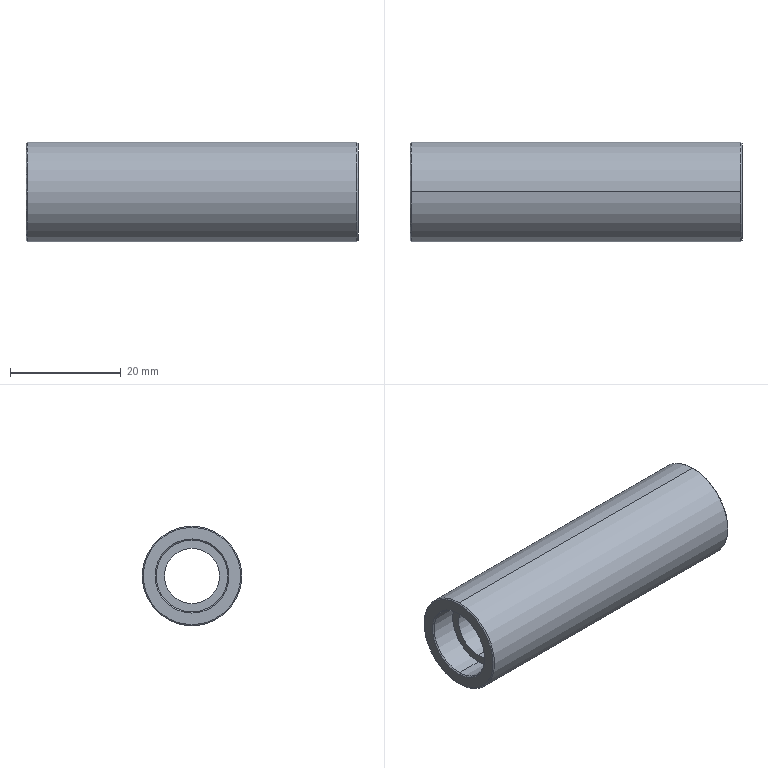Part | SolidWorks | features Chamfer 1, Revolution 1 | 1 solid | 20 faces | box 60 x 18 x 18 mm | volume 10010 mm3 | cone 8 | cylinder 8 | plane 4 | commonest cylinder face diameters 13 x4 10 x2 18 x2
STEP:
#1=CARTESIAN_POINT('',(59.8,0.,6.5));
#2=VERTEX_POINT('',#1);
#3=CARTESIAN_POINT('',(59.8,0.,-6.5));
#4=VERTEX_POINT('',#3);
#5=CARTESIAN_POINT('',(59.8,0.,0.));
#6=DIRECTION('',(1.,0.,0.));
#7=DIRECTION('',(0.,0.,1.));
#8=AXIS2_PLACEMENT_3D('',#5,#6,#7);
#9=CIRCLE('',#8,6.5);
#10=EDGE_CURVE('',#2,#4,#9,.T.);
#11=ORIENTED_EDGE('',*,*,#10,.F.);
#12=CARTESIAN_POINT('',(60.,0.,6.7));
#13=VERTEX_POINT('',#12);
#14=CARTESIAN_POINT('',(60.,0.,6.7));
#15=DIRECTION('',(0.7071,0.,0.7071));
#16=VECTOR('',#15,1000.);
#17=LINE('',#14,#16);
#18=EDGE_CURVE('',#2,#13,#17,.T.);
#19=ORIENTED_EDGE('',*,*,#18,.T.);
#20=CARTESIAN_POINT('',(60.,0.,-6.7));
#21=VERTEX_POINT('',#20);
#22=CARTESIAN_POINT('',(60.,0.,0.));
#23=DIRECTION('',(-1.,0.,0.));
#24=DIRECTION('',(0.,0.,1.));
#25=AXIS2_PLACEMENT_3D('',#22,#23,#24);
#26=CIRCLE('',#25,6.7);
#27=EDGE_CURVE('',#21,#13,#26,.T.);
#28=ORIENTED_EDGE('',*,*,#27,.F.);
#29=CARTESIAN_POINT('',(60.,0.,-6.7));
#30=DIRECTION('',(0.7071,0.,-0.7071));
#31=VECTOR('',#30,1000.);
#32=LINE('',#29,#31);
#33=EDGE_CURVE('',#4,#21,#32,.T.);
#34=ORIENTED_EDGE('',*,*,#33,.F.);
#35=EDGE_LOOP('',(#11,#19,#28,#34));
#36=FACE_OUTER_BOUND('',#35,.T.);
#37=CARTESIAN_POINT('',(60.,0.,0.));
#38=DIRECTION('',(1.,0.,0.));
#39=DIRECTION('',(0.,0.,-1.));
#40=AXIS2_PLACEMENT_3D('',#37,#38,#39);
#41=CONICAL_SURFACE('',#40,6.7,0.7854);
#42=ADVANCED_FACE('',(#36),#41,.F.);
#43=CARTESIAN_POINT('',(60.,0.,-8.8));
#44=VERTEX_POINT('',#43);
#45=CARTESIAN_POINT('',(60.,0.,8.8));
#46=VERTEX_POINT('',#45);
#47=CARTESIAN_POINT('',(60.,0.,0.));
#48=DIRECTION('',(1.,0.,0.));
#49=DIRECTION('',(0.,0.,1.));
#50=AXIS2_PLACEMENT_3D('',#47,#48,#49);
#51=CIRCLE('',#50,8.8);
#52=EDGE_CURVE('',#44,#46,#51,.T.);
#53=ORIENTED_EDGE('',*,*,#52,.F.);
#54=CARTESIAN_POINT('',(59.8,0.,-9.));
#55=VERTEX_POINT('',#54);
#56=CARTESIAN_POINT('',(59.8,0.,-9.));
#57=DIRECTION('',(-0.7071,0.,-0.7071));
#58=VECTOR('',#57,1000.);
#59=LINE('',#56,#58);
#60=EDGE_CURVE('',#44,#55,#59,.T.);
#61=ORIENTED_EDGE('',*,*,#60,.T.);
#62=CARTESIAN_POINT('',(59.8,0.,9.));
#63=VERTEX_POINT('',#62);
#64=CARTESIAN_POINT('',(59.8,0.,0.));
#65=DIRECTION('',(-1.,0.,0.));
#66=DIRECTION('',(0.,0.,1.));
#67=AXIS2_PLACEMENT_3D('',#64,#65,#66);
#68=CIRCLE('',#67,9.);
#69=EDGE_CURVE('',#63,#55,#68,.T.);
#70=ORIENTED_EDGE('',*,*,#69,.F.);
#71=CARTESIAN_POINT('',(59.8,0.,9.));
#72=DIRECTION('',(-0.7071,0.,0.7071));
#73=VECTOR('',#72,1000.);
#74=LINE('',#71,#73);
#75=EDGE_CURVE('',#46,#63,#74,.T.);
#76=ORIENTED_EDGE('',*,*,#75,.F.);
#77=EDGE_LOOP('',(#53,#61,#70,#76));
#78=FACE_OUTER_BOUND('',#77,.T.);
#79=CARTESIAN_POINT('',(59.8,0.,0.));
#80=DIRECTION('',(-1.,0.,0.));
#81=DIRECTION('',(0.,0.,1.));
#82=AXIS2_PLACEMENT_3D('',#79,#80,#81);
#83=CONICAL_SURFACE('',#82,9.,0.7854);
#84=ADVANCED_FACE('',(#78),#83,.T.);
#85=CARTESIAN_POINT('',(0.2,0.,-6.5));
#86=VERTEX_POINT('',#85);
#87=CARTESIAN_POINT('',(0.2,0.,6.5));
#88=VERTEX_POINT('',#87);
#89=CARTESIAN_POINT('',(0.2,0.,0.));
#90=DIRECTION('',(-1.,0.,0.));
#91=DIRECTION('',(0.,0.,-1.));
#92=AXIS2_PLACEMENT_3D('',#89,#90,#91);
#93=CIRCLE('',#92,6.5);
#94=EDGE_CURVE('',#86,#88,#93,.T.);
#95=ORIENTED_EDGE('',*,*,#94,.F.);
#96=CARTESIAN_POINT('',(0.,0.,-6.7));
#97=VERTEX_POINT('',#96);
#98=CARTESIAN_POINT('',(0.2,0.,-6.5));
#99=DIRECTION('',(-0.7071,0.,-0.7071));
#100=VECTOR('',#99,1000.);
#101=LINE('',#98,#100);
#102=EDGE_CURVE('',#86,#97,#101,.T.);
#103=ORIENTED_EDGE('',*,*,#102,.T.);
#104=CARTESIAN_POINT('',(0.,0.,6.7));
#105=VERTEX_POINT('',#104);
#106=CARTESIAN_POINT('',(0.,0.,0.));
#107=DIRECTION('',(1.,0.,0.));
#108=DIRECTION('',(0.,0.,-1.));
#109=AXIS2_PLACEMENT_3D('',#106,#107,#108);
#110=CIRCLE('',#109,6.7);
#111=EDGE_CURVE('',#105,#97,#110,.T.);
#112=ORIENTED_EDGE('',*,*,#111,.F.);
#113=CARTESIAN_POINT('',(0.2,0.,6.5));
#114=DIRECTION('',(-0.7071,0.,0.7071));
#115=VECTOR('',#114,1000.);
#116=LINE('',#113,#115);
#117=EDGE_CURVE('',#88,#105,#116,.T.);
#118=ORIENTED_EDGE('',*,*,#117,.F.);
#119=EDGE_LOOP('',(#95,#103,#112,#118));
#120=FACE_OUTER_BOUND('',#119,.T.);
#121=CARTESIAN_POINT('',(0.2,0.,0.));
#122=DIRECTION('',(-1.,0.,0.));
#123=DIRECTION('',(0.,0.,1.));
#124=AXIS2_PLACEMENT_3D('',#121,#122,#123);
#125=CONICAL_SURFACE('',#124,6.5,0.7854);
#126=ADVANCED_FACE('',(#120),#125,.F.);
#127=CARTESIAN_POINT('',(0.,0.,8.8));
#128=VERTEX_POINT('',#127);
#129=CARTESIAN_POINT('',(0.,0.,-8.8));
#130=VERTEX_POINT('',#129);
#131=CARTESIAN_POINT('',(0.,0.,0.));
#132=DIRECTION('',(-1.,0.,0.));
#133=DIRECTION('',(0.,0.,-1.));
#134=AXIS2_PLACEMENT_3D('',#131,#132,#133);
#135=CIRCLE('',#134,8.8);
#136=EDGE_CURVE('',#128,#130,#135,.T.);
#137=ORIENTED_EDGE('',*,*,#136,.F.);
#138=CARTESIAN_POINT('',(0.2,0.,9.));
#139=VERTEX_POINT('',#138);
#140=CARTESIAN_POINT('',(0.,0.,8.8));
#141=DIRECTION('',(0.7071,0.,0.7071));
#142=VECTOR('',#141,1000.);
#143=LINE('',#140,#142);
#144=EDGE_CURVE('',#128,#139,#143,.T.);
#145=ORIENTED_EDGE('',*,*,#144,.T.);
#146=CARTESIAN_POINT('',(0.2,0.,-9.));
#147=VERTEX_POINT('',#146);
#148=CARTESIAN_POINT('',(0.2,0.,0.));
#149=DIRECTION('',(1.,0.,0.));
#150=DIRECTION('',(0.,0.,-1.));
#151=AXIS2_PLACEMENT_3D('',#148,#149,#150);
#152=CIRCLE('',#151,9.);
#153=EDGE_CURVE('',#147,#139,#152,.T.);
#154=ORIENTED_EDGE('',*,*,#153,.F.);
#155=CARTESIAN_POINT('',(0.,0.,-8.8));
#156=DIRECTION('',(0.7071,0.,-0.7071));
#157=VECTOR('',#156,1000.);
#158=LINE('',#155,#157);
#159=EDGE_CURVE('',#130,#147,#158,.T.);
#160=ORIENTED_EDGE('',*,*,#159,.F.);
#161=EDGE_LOOP('',(#137,#145,#154,#160));
#162=FACE_OUTER_BOUND('',#161,.T.);
#163=CARTESIAN_POINT('',(0.,0.,0.));
#164=DIRECTION('',(1.,0.,0.));
#165=DIRECTION('',(0.,0.,-1.));
#166=AXIS2_PLACEMENT_3D('',#163,#164,#165);
#167=CONICAL_SURFACE('',#166,8.8,0.7854);
#168=ADVANCED_FACE('',(#162),#167,.T.);
#169=CARTESIAN_POINT('',(5.,0.,-6.5));
#170=VERTEX_POINT('',#169);
#171=CARTESIAN_POINT('',(5.,0.,6.5));
#172=VERTEX_POINT('',#171);
#173=CARTESIAN_POINT('',(5.,0.,0.));
#174=DIRECTION('',(-1.,0.,0.));
#175=DIRECTION('',(0.,0.,1.));
#176=AXIS2_PLACEMENT_3D('',#173,#174,#175);
#177=CIRCLE('',#176,6.5);
#178=EDGE_CURVE('',#170,#172,#177,.T.);
#179=ORIENTED_EDGE('',*,*,#178,.F.);
#180=CARTESIAN_POINT('',(0.,0.,-6.5));
#181=DIRECTION('',(-1.,0.,0.));
#182=VECTOR('',#181,1000.);
#183=LINE('',#180,#182);
#184=EDGE_CURVE('',#170,#86,#183,.T.);
#185=ORIENTED_EDGE('',*,*,#184,.T.);
#186=ORIENTED_EDGE('',*,*,#94,.T.);
#187=CARTESIAN_POINT('',(0.,0.,6.5));
#188=DIRECTION('',(-1.,0.,0.));
#189=VECTOR('',#188,1000.);
#190=LINE('',#187,#189);
#191=EDGE_CURVE('',#172,#88,#190,.T.);
#192=ORIENTED_EDGE('',*,*,#191,.F.);
#193=EDGE_LOOP('',(#179,#185,#186,#192));
#194=FACE_OUTER_BOUND('',#193,.T.);
#195=CARTESIAN_POINT('',(0.,0.,0.));
#196=DIRECTION('',(-1.,0.,0.));
#197=DIRECTION('',(0.,0.,1.));
#198=AXIS2_PLACEMENT_3D('',#195,#196,#197);
#199=CYLINDRICAL_SURFACE('',#198,6.5);
#200=ADVANCED_FACE('',(#194),#199,.F.);
#201=CARTESIAN_POINT('',(55.,0.,-5.));
#202=VERTEX_POINT('',#201);
#203=CARTESIAN_POINT('',(55.,0.,5.));
#204=VERTEX_POINT('',#203);
#205=CARTESIAN_POINT('',(55.,0.,0.));
#206=DIRECTION('',(-1.,0.,0.));
#207=DIRECTION('',(0.,0.,1.));
#208=AXIS2_PLACEMENT_3D('',#205,#206,#207);
#209=CIRCLE('',#208,5.);
#210=EDGE_CURVE('',#202,#204,#209,.T.);
#211=ORIENTED_EDGE('',*,*,#210,.F.);
#212=CARTESIAN_POINT('',(5.,0.,-5.));
#213=VERTEX_POINT('',#212);
#214=CARTESIAN_POINT('',(0.,0.,-5.));
#215=DIRECTION('',(-1.,0.,0.));
#216=VECTOR('',#215,1000.);
#217=LINE('',#214,#216);
#218=EDGE_CURVE('',#202,#213,#217,.T.);
#219=ORIENTED_EDGE('',*,*,#218,.T.);
#220=CARTESIAN_POINT('',(5.,0.,5.));
#221=VERTEX_POINT('',#220);
#222=CARTESIAN_POINT('',(5.,0.,0.));
#223=DIRECTION('',(-1.,0.,0.));
#224=DIRECTION('',(0.,0.,1.));
#225=AXIS2_PLACEMENT_3D('',#222,#223,#224);
#226=CIRCLE('',#225,5.);
#227=EDGE_CURVE('',#213,#221,#226,.T.);
#228=ORIENTED_EDGE('',*,*,#227,.T.);
#229=CARTESIAN_POINT('',(0.,0.,5.));
#230=DIRECTION('',(-1.,0.,0.));
#231=VECTOR('',#230,1000.);
#232=LINE('',#229,#231);
#233=EDGE_CURVE('',#204,#221,#232,.T.);
#234=ORIENTED_EDGE('',*,*,#233,.F.);
#235=EDGE_LOOP('',(#211,#219,#228,#234));
#236=FACE_OUTER_BOUND('',#235,.T.);
#237=CARTESIAN_POINT('',(0.,0.,0.));
#238=DIRECTION('',(-1.,0.,0.));
#239=DIRECTION('',(0.,0.,1.));
#240=AXIS2_PLACEMENT_3D('',#237,#238,#239);
#241=CYLINDRICAL_SURFACE('',#240,5.);
#242=ADVANCED_FACE('',(#236),#241,.F.);
#243=ORIENTED_EDGE('',*,*,#10,.T.);
#244=CARTESIAN_POINT('',(55.,0.,-6.5));
#245=VERTEX_POINT('',#244);
#246=CARTESIAN_POINT('',(0.,0.,-6.5));
#247=DIRECTION('',(-1.,0.,0.));
#248=VECTOR('',#247,1000.);
#249=LINE('',#246,#248);
#250=EDGE_CURVE('',#4,#245,#249,.T.);
#251=ORIENTED_EDGE('',*,*,#250,.T.);
#252=CARTESIAN_POINT('',(55.,0.,6.5));
#253=VERTEX_POINT('',#252);
#254=CARTESIAN_POINT('',(55.,0.,0.));
#255=DIRECTION('',(-1.,0.,0.));
#256=DIRECTION('',(0.,0.,1.));
#257=AXIS2_PLACEMENT_3D('',#254,#255,#256);
#258=CIRCLE('',#257,6.5);
#259=EDGE_CURVE('',#245,#253,#258,.T.);
#260=ORIENTED_EDGE('',*,*,#259,.T.);
#261=CARTESIAN_POINT('',(0.,0.,6.5));
#262=DIRECTION('',(-1.,0.,0.));
#263=VECTOR('',#262,1000.);
#264=LINE('',#261,#263);
#265=EDGE_CURVE('',#2,#253,#264,.T.);
#266=ORIENTED_EDGE('',*,*,#265,.F.);
#267=EDGE_LOOP('',(#243,#251,#260,#266));
#268=FACE_OUTER_BOUND('',#267,.T.);
#269=CARTESIAN_POINT('',(0.,0.,0.));
#270=DIRECTION('',(-1.,0.,0.));
#271=DIRECTION('',(0.,0.,1.));
#272=AXIS2_PLACEMENT_3D('',#269,#270,#271);
#273=CYLINDRICAL_SURFACE('',#272,6.5);
#274=ADVANCED_FACE('',(#268),#273,.F.);
#275=ORIENTED_EDGE('',*,*,#69,.T.);
#276=CARTESIAN_POINT('',(0.,0.,-9.));
#277=DIRECTION('',(-1.,0.,0.));
#278=VECTOR('',#277,1000.);
#279=LINE('',#276,#278);
#280=EDGE_CURVE('',#55,#147,#279,.T.);
#281=ORIENTED_EDGE('',*,*,#280,.T.);
#282=ORIENTED_EDGE('',*,*,#153,.T.);
#283=CARTESIAN_POINT('',(0.,0.,9.));
#284=DIRECTION('',(-1.,0.,0.));
#285=VECTOR('',#284,1000.);
#286=LINE('',#283,#285);
#287=EDGE_CURVE('',#63,#139,#286,.T.);
#288=ORIENTED_EDGE('',*,*,#287,.F.);
#289=EDGE_LOOP('',(#275,#281,#282,#288));
#290=FACE_OUTER_BOUND('',#289,.T.);
#291=CARTESIAN_POINT('',(0.,0.,0.));
#292=DIRECTION('',(-1.,0.,0.));
#293=DIRECTION('',(0.,0.,1.));
#294=AXIS2_PLACEMENT_3D('',#291,#292,#293);
#295=CYLINDRICAL_SURFACE('',#294,9.);
#296=ADVANCED_FACE('',(#290),#295,.T.);
#297=CARTESIAN_POINT('',(0.,0.,0.));
#298=DIRECTION('',(-1.,0.,0.));
#299=DIRECTION('',(0.,0.,-1.));
#300=AXIS2_PLACEMENT_3D('',#297,#298,#299);
#301=CIRCLE('',#300,8.8);
#302=EDGE_CURVE('',#130,#128,#301,.T.);
#303=ORIENTED_EDGE('',*,*,#302,.T.);
#304=ORIENTED_EDGE('',*,*,#136,.T.);
#305=EDGE_LOOP('',(#303,#304));
#306=FACE_OUTER_BOUND('',#305,.T.);
#307=ORIENTED_EDGE('',*,*,#111,.T.);
#308=CARTESIAN_POINT('',(0.,0.,0.));
#309=DIRECTION('',(1.,0.,0.));
#310=DIRECTION('',(0.,0.,-1.));
#311=AXIS2_PLACEMENT_3D('',#308,#309,#310);
#312=CIRCLE('',#311,6.7);
#313=EDGE_CURVE('',#97,#105,#312,.T.);
#314=ORIENTED_EDGE('',*,*,#313,.T.);
#315=EDGE_LOOP('',(#307,#314));
#316=FACE_BOUND('',#315,.T.);
#317=CARTESIAN_POINT('',(0.,6.5,0.));
#318=DIRECTION('',(1.,0.,0.));
#319=DIRECTION('',(0.,0.,-1.));
#320=AXIS2_PLACEMENT_3D('',#317,#318,#319);
#321=PLANE('',#320);
#322=ADVANCED_FACE('',(#306,#316),#321,.F.);
#323=ORIENTED_EDGE('',*,*,#280,.F.);
#324=CARTESIAN_POINT('',(59.8,0.,0.));
#325=DIRECTION('',(-1.,0.,0.));
#326=DIRECTION('',(0.,0.,1.));
#327=AXIS2_PLACEMENT_3D('',#324,#325,#326);
#328=CIRCLE('',#327,9.);
#329=EDGE_CURVE('',#55,#63,#328,.T.);
#330=ORIENTED_EDGE('',*,*,#329,.T.);
#331=ORIENTED_EDGE('',*,*,#287,.T.);
#332=CARTESIAN_POINT('',(0.2,0.,0.));
#333=DIRECTION('',(1.,0.,0.));
#334=DIRECTION('',(0.,0.,-1.));
#335=AXIS2_PLACEMENT_3D('',#332,#333,#334);
#336=CIRCLE('',#335,9.);
#337=EDGE_CURVE('',#139,#147,#336,.T.);
#338=ORIENTED_EDGE('',*,*,#337,.T.);
#339=EDGE_LOOP('',(#323,#330,#331,#338));
#340=FACE_OUTER_BOUND('',#339,.T.);
#341=CARTESIAN_POINT('',(0.,0.,0.));
#342=DIRECTION('',(-1.,0.,0.));
#343=DIRECTION('',(0.,0.,1.));
#344=AXIS2_PLACEMENT_3D('',#341,#342,#343);
#345=CYLINDRICAL_SURFACE('',#344,9.);
#346=ADVANCED_FACE('',(#340),#345,.T.);
#347=CARTESIAN_POINT('',(60.,0.,0.));
#348=DIRECTION('',(1.,0.,0.));
#349=DIRECTION('',(0.,0.,1.));
#350=AXIS2_PLACEMENT_3D('',#347,#348,#349);
#351=CIRCLE('',#350,8.8);
#352=EDGE_CURVE('',#46,#44,#351,.T.);
#353=ORIENTED_EDGE('',*,*,#352,.T.);
#354=ORIENTED_EDGE('',*,*,#52,.T.);
#355=EDGE_LOOP('',(#353,#354));
#356=FACE_OUTER_BOUND('',#355,.T.);
#357=ORIENTED_EDGE('',*,*,#27,.T.);
#358=CARTESIAN_POINT('',(60.,0.,0.));
#359=DIRECTION('',(-1.,0.,0.));
#360=DIRECTION('',(0.,0.,1.));
#361=AXIS2_PLACEMENT_3D('',#358,#359,#360);
#362=CIRCLE('',#361,6.7);
#363=EDGE_CURVE('',#13,#21,#362,.T.);
#364=ORIENTED_EDGE('',*,*,#363,.T.);
#365=EDGE_LOOP('',(#357,#364));
#366=FACE_BOUND('',#365,.T.);
#367=CARTESIAN_POINT('',(60.,9.,0.));
#368=DIRECTION('',(-1.,0.,0.));
#369=DIRECTION('',(0.,0.,1.));
#370=AXIS2_PLACEMENT_3D('',#367,#368,#369);
#371=PLANE('',#370);
#372=ADVANCED_FACE('',(#356,#366),#371,.F.);
#373=ORIENTED_EDGE('',*,*,#250,.F.);
#374=CARTESIAN_POINT('',(59.8,0.,0.));
#375=DIRECTION('',(1.,0.,0.));
#376=DIRECTION('',(0.,0.,1.));
#377=AXIS2_PLACEMENT_3D('',#374,#375,#376);
#378=CIRCLE('',#377,6.5);
#379=EDGE_CURVE('',#4,#2,#378,.T.);
#380=ORIENTED_EDGE('',*,*,#379,.T.);
#381=ORIENTED_EDGE('',*,*,#265,.T.);
#382=CARTESIAN_POINT('',(55.,0.,0.));
#383=DIRECTION('',(-1.,0.,0.));
#384=DIRECTION('',(0.,0.,1.));
#385=AXIS2_PLACEMENT_3D('',#382,#383,#384);
#386=CIRCLE('',#385,6.5);
#387=EDGE_CURVE('',#253,#245,#386,.T.);
#388=ORIENTED_EDGE('',*,*,#387,.T.);
#389=EDGE_LOOP('',(#373,#380,#381,#388));
#390=FACE_OUTER_BOUND('',#389,.T.);
#391=CARTESIAN_POINT('',(0.,0.,0.));
#392=DIRECTION('',(-1.,0.,0.));
#393=DIRECTION('',(0.,0.,1.));
#394=AXIS2_PLACEMENT_3D('',#391,#392,#393);
#395=CYLINDRICAL_SURFACE('',#394,6.5);
#396=ADVANCED_FACE('',(#390),#395,.F.);
#397=ORIENTED_EDGE('',*,*,#387,.F.);
#398=ORIENTED_EDGE('',*,*,#259,.F.);
#399=EDGE_LOOP('',(#397,#398));
#400=FACE_OUTER_BOUND('',#399,.T.);
#401=CARTESIAN_POINT('',(55.,0.,0.));
#402=DIRECTION('',(-1.,0.,0.));
#403=DIRECTION('',(0.,0.,1.));
#404=AXIS2_PLACEMENT_3D('',#401,#402,#403);
#405=CIRCLE('',#404,5.);
#406=EDGE_CURVE('',#204,#202,#405,.T.);
#407=ORIENTED_EDGE('',*,*,#406,.T.);
#408=ORIENTED_EDGE('',*,*,#210,.T.);
#409=EDGE_LOOP('',(#407,#408));
#410=FACE_BOUND('',#409,.T.);
#411=CARTESIAN_POINT('',(55.,6.5,0.));
#412=DIRECTION('',(-1.,0.,0.));
#413=DIRECTION('',(0.,0.,1.));
#414=AXIS2_PLACEMENT_3D('',#411,#412,#413);
#415=PLANE('',#414);
#416=ADVANCED_FACE('',(#400,#410),#415,.F.);
#417=ORIENTED_EDGE('',*,*,#218,.F.);
#418=ORIENTED_EDGE('',*,*,#406,.F.);
#419=ORIENTED_EDGE('',*,*,#233,.T.);
#420=CARTESIAN_POINT('',(5.,0.,0.));
#421=DIRECTION('',(-1.,0.,0.));
#422=DIRECTION('',(0.,0.,1.));
#423=AXIS2_PLACEMENT_3D('',#420,#421,#422);
#424=CIRCLE('',#423,5.);
#425=EDGE_CURVE('',#221,#213,#424,.T.);
#426=ORIENTED_EDGE('',*,*,#425,.T.);
#427=EDGE_LOOP('',(#417,#418,#419,#426));
#428=FACE_OUTER_BOUND('',#427,.T.);
#429=CARTESIAN_POINT('',(0.,0.,0.));
#430=DIRECTION('',(-1.,0.,0.));
#431=DIRECTION('',(0.,0.,1.));
#432=AXIS2_PLACEMENT_3D('',#429,#430,#431);
#433=CYLINDRICAL_SURFACE('',#432,5.);
#434=ADVANCED_FACE('',(#428),#433,.F.);
#435=ORIENTED_EDGE('',*,*,#425,.F.);
#436=ORIENTED_EDGE('',*,*,#227,.F.);
#437=EDGE_LOOP('',(#435,#436));
#438=FACE_BOUND('',#437,.T.);
#439=CARTESIAN_POINT('',(5.,0.,0.));
#440=DIRECTION('',(-1.,0.,0.));
#441=DIRECTION('',(0.,0.,1.));
#442=AXIS2_PLACEMENT_3D('',#439,#440,#441);
#443=CIRCLE('',#442,6.5);
#444=EDGE_CURVE('',#172,#170,#443,.T.);
#445=ORIENTED_EDGE('',*,*,#444,.T.);
#446=ORIENTED_EDGE('',*,*,#178,.T.);
#447=EDGE_LOOP('',(#445,#446));
#448=FACE_OUTER_BOUND('',#447,.T.);
#449=CARTESIAN_POINT('',(5.,5.,0.));
#450=DIRECTION('',(1.,0.,0.));
#451=DIRECTION('',(0.,0.,-1.));
#452=AXIS2_PLACEMENT_3D('',#449,#450,#451);
#453=PLANE('',#452);
#454=ADVANCED_FACE('',(#438,#448),#453,.F.);
#455=ORIENTED_EDGE('',*,*,#184,.F.);
#456=ORIENTED_EDGE('',*,*,#444,.F.);
#457=ORIENTED_EDGE('',*,*,#191,.T.);
#458=CARTESIAN_POINT('',(0.2,0.,0.));
#459=DIRECTION('',(-1.,0.,0.));
#460=DIRECTION('',(0.,0.,-1.));
#461=AXIS2_PLACEMENT_3D('',#458,#459,#460);
#462=CIRCLE('',#461,6.5);
#463=EDGE_CURVE('',#88,#86,#462,.T.);
#464=ORIENTED_EDGE('',*,*,#463,.T.);
#465=EDGE_LOOP('',(#455,#456,#457,#464));
#466=FACE_OUTER_BOUND('',#465,.T.);
#467=CARTESIAN_POINT('',(0.,0.,0.));
#468=DIRECTION('',(-1.,0.,0.));
#469=DIRECTION('',(0.,0.,1.));
#470=AXIS2_PLACEMENT_3D('',#467,#468,#469);
#471=CYLINDRICAL_SURFACE('',#470,6.5);
#472=ADVANCED_FACE('',(#466),#471,.F.);
#473=ORIENTED_EDGE('',*,*,#144,.F.);
#474=ORIENTED_EDGE('',*,*,#302,.F.);
#475=ORIENTED_EDGE('',*,*,#159,.T.);
#476=ORIENTED_EDGE('',*,*,#337,.F.);
#477=EDGE_LOOP('',(#473,#474,#475,#476));
#478=FACE_OUTER_BOUND('',#477,.T.);
#479=CARTESIAN_POINT('',(0.,0.,0.));
#480=DIRECTION('',(1.,0.,0.));
#481=DIRECTION('',(0.,0.,-1.));
#482=AXIS2_PLACEMENT_3D('',#479,#480,#481);
#483=CONICAL_SURFACE('',#482,8.8,0.7854);
#484=ADVANCED_FACE('',(#478),#483,.T.);
#485=ORIENTED_EDGE('',*,*,#102,.F.);
#486=ORIENTED_EDGE('',*,*,#463,.F.);
#487=ORIENTED_EDGE('',*,*,#117,.T.);
#488=ORIENTED_EDGE('',*,*,#313,.F.);
#489=EDGE_LOOP('',(#485,#486,#487,#488));
#490=FACE_OUTER_BOUND('',#489,.T.);
#491=CARTESIAN_POINT('',(0.2,0.,0.));
#492=DIRECTION('',(-1.,0.,0.));
#493=DIRECTION('',(0.,0.,1.));
#494=AXIS2_PLACEMENT_3D('',#491,#492,#493);
#495=CONICAL_SURFACE('',#494,6.5,0.7854);
#496=ADVANCED_FACE('',(#490),#495,.F.);
#497=ORIENTED_EDGE('',*,*,#60,.F.);
#498=ORIENTED_EDGE('',*,*,#352,.F.);
#499=ORIENTED_EDGE('',*,*,#75,.T.);
#500=ORIENTED_EDGE('',*,*,#329,.F.);
#501=EDGE_LOOP('',(#497,#498,#499,#500));
#502=FACE_OUTER_BOUND('',#501,.T.);
#503=CARTESIAN_POINT('',(59.8,0.,0.));
#504=DIRECTION('',(-1.,0.,0.));
#505=DIRECTION('',(0.,0.,1.));
#506=AXIS2_PLACEMENT_3D('',#503,#504,#505);
#507=CONICAL_SURFACE('',#506,9.,0.7854);
#508=ADVANCED_FACE('',(#502),#507,.T.);
#509=ORIENTED_EDGE('',*,*,#18,.F.);
#510=ORIENTED_EDGE('',*,*,#379,.F.);
#511=ORIENTED_EDGE('',*,*,#33,.T.);
#512=ORIENTED_EDGE('',*,*,#363,.F.);
#513=EDGE_LOOP('',(#509,#510,#511,#512));
#514=FACE_OUTER_BOUND('',#513,.T.);
#515=CARTESIAN_POINT('',(60.,0.,0.));
#516=DIRECTION('',(1.,0.,0.));
#517=DIRECTION('',(0.,0.,-1.));
#518=AXIS2_PLACEMENT_3D('',#515,#516,#517);
#519=CONICAL_SURFACE('',#518,6.7,0.7854);
#520=ADVANCED_FACE('',(#514),#519,.F.);
#521=CLOSED_SHELL('',(#42,#84,#126,#168,#200,#242,#274,#296,#322,#346,#372,#396,#416,#434,#454,#472,#484,#496,#508,#520));
#522=MANIFOLD_SOLID_BREP('',#521);
#523=CARTESIAN_POINT('',(0.,0.,0.));
#524=DIRECTION('',(0.,0.,1.));
#525=DIRECTION('',(1.,0.,0.));
#526=AXIS2_PLACEMENT_3D('',#523,#524,#525);
#527=(LENGTH_UNIT()NAMED_UNIT(*)SI_UNIT(.MILLI.,.METRE.));
#528=UNCERTAINTY_MEASURE_WITH_UNIT(LENGTH_MEASURE(0.00001),#527,'','');
#529=(NAMED_UNIT(*)PLANE_ANGLE_UNIT()SI_UNIT($,.RADIAN.));
#530=(NAMED_UNIT(*)SI_UNIT($,.STERADIAN.)SOLID_ANGLE_UNIT());
#531=(GEOMETRIC_REPRESENTATION_CONTEXT(3)GLOBAL_UNCERTAINTY_ASSIGNED_CONTEXT((#528))GLOBAL_UNIT_ASSIGNED_CONTEXT((#527,#529,#530))REPRESENTATION_CONTEXT('',''));
#532=ADVANCED_BREP_SHAPE_REPRESENTATION('',(#522,#526),#531);